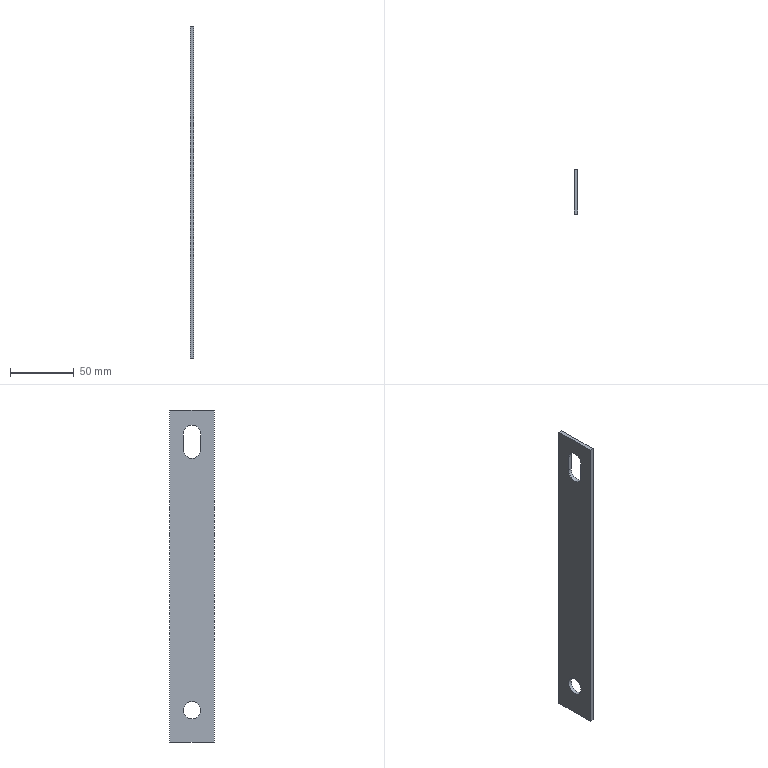Part | NX | features solid 2 | 1 solid | 11 faces | box 3 x 35 x 260 mm | volume 25935 mm3 | plane 8 | cylinder 3 | commonest cylinder face diameters 13.5 x3
STEP:
#1=CARTESIAN_POINT('',(1230.,-511.75,76.25));
#2=VERTEX_POINT('',#1);
#3=CARTESIAN_POINT('',(1230.,-498.25,76.25));
#4=VERTEX_POINT('',#3);
#5=CARTESIAN_POINT('',(1230.,-505.,76.25));
#6=DIRECTION('',(-1.,0.,0.));
#7=DIRECTION('',(0.,-1.,0.));
#8=AXIS2_PLACEMENT_3D('',#5,#6,#7);
#9=CIRCLE('',#8,6.75);
#10=EDGE_CURVE('',#2,#4,#9,.T.);
#11=ORIENTED_EDGE('',*,*,#10,.T.);
#12=CARTESIAN_POINT('',(1233.,-498.25,76.25));
#13=VERTEX_POINT('',#12);
#14=CARTESIAN_POINT('',(1233.,-498.25,76.25));
#15=DIRECTION('',(-1.,0.,0.));
#16=VECTOR('',#15,1000.);
#17=LINE('',#14,#16);
#18=EDGE_CURVE('',#13,#4,#17,.T.);
#19=ORIENTED_EDGE('',*,*,#18,.F.);
#20=CARTESIAN_POINT('',(1233.,-511.75,76.25));
#21=VERTEX_POINT('',#20);
#22=CARTESIAN_POINT('',(1233.,-505.,76.25));
#23=DIRECTION('',(-1.,0.,0.));
#24=DIRECTION('',(0.,-1.,0.));
#25=AXIS2_PLACEMENT_3D('',#22,#23,#24);
#26=CIRCLE('',#25,6.75);
#27=EDGE_CURVE('',#21,#13,#26,.T.);
#28=ORIENTED_EDGE('',*,*,#27,.F.);
#29=CARTESIAN_POINT('',(1233.,-511.75,76.25));
#30=DIRECTION('',(-1.,0.,0.));
#31=VECTOR('',#30,1000.);
#32=LINE('',#29,#31);
#33=EDGE_CURVE('',#21,#2,#32,.T.);
#34=ORIENTED_EDGE('',*,*,#33,.T.);
#35=EDGE_LOOP('',(#11,#19,#28,#34));
#36=FACE_BOUND('',#35,.T.);
#37=CARTESIAN_POINT('',(1233.,-505.,76.25));
#38=DIRECTION('',(-1.,0.,0.));
#39=DIRECTION('',(0.,-1.,0.));
#40=AXIS2_PLACEMENT_3D('',#37,#38,#39);
#41=CYLINDRICAL_SURFACE('',#40,6.75);
#42=ADVANCED_FACE('',(#36),#41,.F.);
#43=CARTESIAN_POINT('',(1230.,-511.75,63.75));
#44=VERTEX_POINT('',#43);
#45=CARTESIAN_POINT('',(1230.,-511.75,76.25));
#46=DIRECTION('',(0.,0.,-1.));
#47=VECTOR('',#46,1000.);
#48=LINE('',#45,#47);
#49=EDGE_CURVE('',#2,#44,#48,.T.);
#50=ORIENTED_EDGE('',*,*,#49,.F.);
#51=ORIENTED_EDGE('',*,*,#33,.F.);
#52=CARTESIAN_POINT('',(1233.,-511.75,63.75));
#53=VERTEX_POINT('',#52);
#54=CARTESIAN_POINT('',(1233.,-511.75,76.25));
#55=DIRECTION('',(0.,0.,-1.));
#56=VECTOR('',#55,1000.);
#57=LINE('',#54,#56);
#58=EDGE_CURVE('',#21,#53,#57,.T.);
#59=ORIENTED_EDGE('',*,*,#58,.T.);
#60=CARTESIAN_POINT('',(1233.,-511.75,63.75));
#61=DIRECTION('',(-1.,0.,0.));
#62=VECTOR('',#61,1000.);
#63=LINE('',#60,#62);
#64=EDGE_CURVE('',#53,#44,#63,.T.);
#65=ORIENTED_EDGE('',*,*,#64,.T.);
#66=EDGE_LOOP('',(#50,#51,#59,#65));
#67=FACE_BOUND('',#66,.T.);
#68=CARTESIAN_POINT('',(1233.,-511.75,76.25));
#69=DIRECTION('',(0.,1.,0.));
#70=DIRECTION('',(-1.,0.,0.));
#71=AXIS2_PLACEMENT_3D('',#68,#69,#70);
#72=PLANE('',#71);
#73=ADVANCED_FACE('',(#67),#72,.T.);
#74=CARTESIAN_POINT('',(1230.,-498.25,63.75));
#75=VERTEX_POINT('',#74);
#76=CARTESIAN_POINT('',(1230.,-505.,63.75));
#77=DIRECTION('',(-1.,0.,0.));
#78=DIRECTION('',(0.,-1.,0.));
#79=AXIS2_PLACEMENT_3D('',#76,#77,#78);
#80=CIRCLE('',#79,6.75);
#81=EDGE_CURVE('',#75,#44,#80,.T.);
#82=ORIENTED_EDGE('',*,*,#81,.T.);
#83=ORIENTED_EDGE('',*,*,#64,.F.);
#84=CARTESIAN_POINT('',(1233.,-498.25,63.75));
#85=VERTEX_POINT('',#84);
#86=CARTESIAN_POINT('',(1233.,-505.,63.75));
#87=DIRECTION('',(-1.,0.,0.));
#88=DIRECTION('',(0.,-1.,0.));
#89=AXIS2_PLACEMENT_3D('',#86,#87,#88);
#90=CIRCLE('',#89,6.75);
#91=EDGE_CURVE('',#85,#53,#90,.T.);
#92=ORIENTED_EDGE('',*,*,#91,.F.);
#93=CARTESIAN_POINT('',(1233.,-498.25,63.75));
#94=DIRECTION('',(-1.,0.,0.));
#95=VECTOR('',#94,1000.);
#96=LINE('',#93,#95);
#97=EDGE_CURVE('',#85,#75,#96,.T.);
#98=ORIENTED_EDGE('',*,*,#97,.T.);
#99=EDGE_LOOP('',(#82,#83,#92,#98));
#100=FACE_BOUND('',#99,.T.);
#101=CARTESIAN_POINT('',(1233.,-505.,63.75));
#102=DIRECTION('',(-1.,0.,0.));
#103=DIRECTION('',(0.,-1.,0.));
#104=AXIS2_PLACEMENT_3D('',#101,#102,#103);
#105=CYLINDRICAL_SURFACE('',#104,6.75);
#106=ADVANCED_FACE('',(#100),#105,.F.);
#107=CARTESIAN_POINT('',(1230.,-522.5,-165.));
#108=VERTEX_POINT('',#107);
#109=CARTESIAN_POINT('',(1230.,-522.5,95.));
#110=VERTEX_POINT('',#109);
#111=CARTESIAN_POINT('',(1230.,-522.5,-205.));
#112=DIRECTION('',(0.,0.,1.));
#113=VECTOR('',#112,1000.);
#114=LINE('',#111,#113);
#115=EDGE_CURVE('',#108,#110,#114,.T.);
#116=ORIENTED_EDGE('',*,*,#115,.F.);
#117=CARTESIAN_POINT('',(1233.,-522.5,-165.));
#118=VERTEX_POINT('',#117);
#119=CARTESIAN_POINT('',(1233.,-522.5,-165.));
#120=DIRECTION('',(-1.,0.,0.));
#121=VECTOR('',#120,1000.);
#122=LINE('',#119,#121);
#123=EDGE_CURVE('',#118,#108,#122,.T.);
#124=ORIENTED_EDGE('',*,*,#123,.F.);
#125=CARTESIAN_POINT('',(1233.,-522.5,95.));
#126=VERTEX_POINT('',#125);
#127=CARTESIAN_POINT('',(1233.,-522.5,-205.));
#128=DIRECTION('',(0.,0.,1.));
#129=VECTOR('',#128,1000.);
#130=LINE('',#127,#129);
#131=EDGE_CURVE('',#118,#126,#130,.T.);
#132=ORIENTED_EDGE('',*,*,#131,.T.);
#133=CARTESIAN_POINT('',(1233.,-522.5,95.));
#134=DIRECTION('',(-1.,0.,0.));
#135=VECTOR('',#134,1000.);
#136=LINE('',#133,#135);
#137=EDGE_CURVE('',#126,#110,#136,.T.);
#138=ORIENTED_EDGE('',*,*,#137,.T.);
#139=EDGE_LOOP('',(#116,#124,#132,#138));
#140=FACE_BOUND('',#139,.T.);
#141=CARTESIAN_POINT('',(1233.,-522.5,-205.));
#142=DIRECTION('',(0.,-1.,0.));
#143=DIRECTION('',(0.,0.,1.));
#144=AXIS2_PLACEMENT_3D('',#141,#142,#143);
#145=PLANE('',#144);
#146=ADVANCED_FACE('',(#140),#145,.T.);
#147=CARTESIAN_POINT('',(1230.,-487.5,95.));
#148=VERTEX_POINT('',#147);
#149=CARTESIAN_POINT('',(1230.,-522.5,95.));
#150=DIRECTION('',(0.,1.,0.));
#151=VECTOR('',#150,1000.);
#152=LINE('',#149,#151);
#153=EDGE_CURVE('',#110,#148,#152,.T.);
#154=ORIENTED_EDGE('',*,*,#153,.F.);
#155=ORIENTED_EDGE('',*,*,#137,.F.);
#156=CARTESIAN_POINT('',(1233.,-487.5,95.));
#157=VERTEX_POINT('',#156);
#158=CARTESIAN_POINT('',(1233.,-522.5,95.));
#159=DIRECTION('',(0.,1.,0.));
#160=VECTOR('',#159,1000.);
#161=LINE('',#158,#160);
#162=EDGE_CURVE('',#126,#157,#161,.T.);
#163=ORIENTED_EDGE('',*,*,#162,.T.);
#164=CARTESIAN_POINT('',(1233.,-487.5,95.));
#165=DIRECTION('',(-1.,0.,0.));
#166=VECTOR('',#165,1000.);
#167=LINE('',#164,#166);
#168=EDGE_CURVE('',#157,#148,#167,.T.);
#169=ORIENTED_EDGE('',*,*,#168,.T.);
#170=EDGE_LOOP('',(#154,#155,#163,#169));
#171=FACE_BOUND('',#170,.T.);
#172=CARTESIAN_POINT('',(1233.,-522.5,95.));
#173=DIRECTION('',(0.,0.,1.));
#174=DIRECTION('',(-1.,0.,0.));
#175=AXIS2_PLACEMENT_3D('',#172,#173,#174);
#176=PLANE('',#175);
#177=ADVANCED_FACE('',(#171),#176,.T.);
#178=CARTESIAN_POINT('',(1230.,-487.5,-165.));
#179=VERTEX_POINT('',#178);
#180=CARTESIAN_POINT('',(1230.,-487.5,95.));
#181=DIRECTION('',(0.,0.,-1.));
#182=VECTOR('',#181,1000.);
#183=LINE('',#180,#182);
#184=EDGE_CURVE('',#148,#179,#183,.T.);
#185=ORIENTED_EDGE('',*,*,#184,.F.);
#186=ORIENTED_EDGE('',*,*,#168,.F.);
#187=CARTESIAN_POINT('',(1233.,-487.5,-165.));
#188=VERTEX_POINT('',#187);
#189=CARTESIAN_POINT('',(1233.,-487.5,95.));
#190=DIRECTION('',(0.,0.,-1.));
#191=VECTOR('',#190,1000.);
#192=LINE('',#189,#191);
#193=EDGE_CURVE('',#157,#188,#192,.T.);
#194=ORIENTED_EDGE('',*,*,#193,.T.);
#195=CARTESIAN_POINT('',(1233.,-487.5,-165.));
#196=DIRECTION('',(-1.,0.,0.));
#197=VECTOR('',#196,1000.);
#198=LINE('',#195,#197);
#199=EDGE_CURVE('',#188,#179,#198,.T.);
#200=ORIENTED_EDGE('',*,*,#199,.T.);
#201=EDGE_LOOP('',(#185,#186,#194,#200));
#202=FACE_BOUND('',#201,.T.);
#203=CARTESIAN_POINT('',(1233.,-487.5,95.));
#204=DIRECTION('',(0.,1.,0.));
#205=DIRECTION('',(0.,0.,-1.));
#206=AXIS2_PLACEMENT_3D('',#203,#204,#205);
#207=PLANE('',#206);
#208=ADVANCED_FACE('',(#202),#207,.T.);
#209=CARTESIAN_POINT('',(1233.,-511.75,-140.));
#210=VERTEX_POINT('',#209);
#211=CARTESIAN_POINT('',(1233.,-505.,-140.));
#212=DIRECTION('',(-1.,0.,0.));
#213=DIRECTION('',(0.,-1.,0.));
#214=AXIS2_PLACEMENT_3D('',#211,#212,#213);
#215=CIRCLE('',#214,6.75);
#216=EDGE_CURVE('',#210,#210,#215,.T.);
#217=ORIENTED_EDGE('',*,*,#216,.F.);
#218=EDGE_LOOP('',(#217));
#219=FACE_BOUND('',#218,.T.);
#220=CARTESIAN_POINT('',(1230.,-511.75,-140.));
#221=VERTEX_POINT('',#220);
#222=CARTESIAN_POINT('',(1230.,-505.,-140.));
#223=DIRECTION('',(-1.,0.,0.));
#224=DIRECTION('',(0.,-1.,0.));
#225=AXIS2_PLACEMENT_3D('',#222,#223,#224);
#226=CIRCLE('',#225,6.75);
#227=EDGE_CURVE('',#221,#221,#226,.T.);
#228=ORIENTED_EDGE('',*,*,#227,.T.);
#229=EDGE_LOOP('',(#228));
#230=FACE_BOUND('',#229,.T.);
#231=CARTESIAN_POINT('',(1233.,-505.,-140.));
#232=DIRECTION('',(-1.,0.,0.));
#233=DIRECTION('',(0.,-1.,0.));
#234=AXIS2_PLACEMENT_3D('',#231,#232,#233);
#235=CYLINDRICAL_SURFACE('',#234,6.75);
#236=ADVANCED_FACE('',(#219,#230),#235,.F.);
#237=CARTESIAN_POINT('',(1230.,-522.5,-165.));
#238=DIRECTION('',(0.,-1.,0.));
#239=VECTOR('',#238,1000.);
#240=LINE('',#237,#239);
#241=EDGE_CURVE('',#179,#108,#240,.T.);
#242=ORIENTED_EDGE('',*,*,#241,.F.);
#243=ORIENTED_EDGE('',*,*,#199,.F.);
#244=CARTESIAN_POINT('',(1233.,-522.5,-165.));
#245=DIRECTION('',(0.,-1.,0.));
#246=VECTOR('',#245,1000.);
#247=LINE('',#244,#246);
#248=EDGE_CURVE('',#188,#118,#247,.T.);
#249=ORIENTED_EDGE('',*,*,#248,.T.);
#250=ORIENTED_EDGE('',*,*,#123,.T.);
#251=EDGE_LOOP('',(#242,#243,#249,#250));
#252=FACE_BOUND('',#251,.T.);
#253=CARTESIAN_POINT('',(1233.,-487.5,-165.));
#254=DIRECTION('',(0.,0.,-1.));
#255=DIRECTION('',(1.,0.,0.));
#256=AXIS2_PLACEMENT_3D('',#253,#254,#255);
#257=PLANE('',#256);
#258=ADVANCED_FACE('',(#252),#257,.T.);
#259=CARTESIAN_POINT('',(1230.,-498.25,63.75));
#260=DIRECTION('',(0.,0.,1.));
#261=VECTOR('',#260,1000.);
#262=LINE('',#259,#261);
#263=EDGE_CURVE('',#75,#4,#262,.T.);
#264=ORIENTED_EDGE('',*,*,#263,.F.);
#265=ORIENTED_EDGE('',*,*,#97,.F.);
#266=CARTESIAN_POINT('',(1233.,-498.25,63.75));
#267=DIRECTION('',(0.,0.,1.));
#268=VECTOR('',#267,1000.);
#269=LINE('',#266,#268);
#270=EDGE_CURVE('',#85,#13,#269,.T.);
#271=ORIENTED_EDGE('',*,*,#270,.T.);
#272=ORIENTED_EDGE('',*,*,#18,.T.);
#273=EDGE_LOOP('',(#264,#265,#271,#272));
#274=FACE_BOUND('',#273,.T.);
#275=CARTESIAN_POINT('',(1233.,-498.25,63.75));
#276=DIRECTION('',(0.,-1.,0.));
#277=DIRECTION('',(1.,0.,0.));
#278=AXIS2_PLACEMENT_3D('',#275,#276,#277);
#279=PLANE('',#278);
#280=ADVANCED_FACE('',(#274),#279,.T.);
#281=ORIENTED_EDGE('',*,*,#131,.F.);
#282=ORIENTED_EDGE('',*,*,#248,.F.);
#283=ORIENTED_EDGE('',*,*,#193,.F.);
#284=ORIENTED_EDGE('',*,*,#162,.F.);
#285=EDGE_LOOP('',(#281,#282,#283,#284));
#286=FACE_BOUND('',#285,.T.);
#287=ORIENTED_EDGE('',*,*,#216,.T.);
#288=EDGE_LOOP('',(#287));
#289=FACE_BOUND('',#288,.T.);
#290=ORIENTED_EDGE('',*,*,#27,.T.);
#291=ORIENTED_EDGE('',*,*,#270,.F.);
#292=ORIENTED_EDGE('',*,*,#91,.T.);
#293=ORIENTED_EDGE('',*,*,#58,.F.);
#294=EDGE_LOOP('',(#290,#291,#292,#293));
#295=FACE_BOUND('',#294,.T.);
#296=CARTESIAN_POINT('',(1233.,-522.5,95.));
#297=DIRECTION('',(-1.,0.,0.));
#298=DIRECTION('',(0.,-1.,0.));
#299=AXIS2_PLACEMENT_3D('',#296,#297,#298);
#300=PLANE('',#299);
#301=ADVANCED_FACE('',(#286,#289,#295),#300,.F.);
#302=ORIENTED_EDGE('',*,*,#115,.T.);
#303=ORIENTED_EDGE('',*,*,#153,.T.);
#304=ORIENTED_EDGE('',*,*,#184,.T.);
#305=ORIENTED_EDGE('',*,*,#241,.T.);
#306=EDGE_LOOP('',(#302,#303,#304,#305));
#307=FACE_BOUND('',#306,.T.);
#308=ORIENTED_EDGE('',*,*,#227,.F.);
#309=EDGE_LOOP('',(#308));
#310=FACE_BOUND('',#309,.T.);
#311=ORIENTED_EDGE('',*,*,#10,.F.);
#312=ORIENTED_EDGE('',*,*,#49,.T.);
#313=ORIENTED_EDGE('',*,*,#81,.F.);
#314=ORIENTED_EDGE('',*,*,#263,.T.);
#315=EDGE_LOOP('',(#311,#312,#313,#314));
#316=FACE_BOUND('',#315,.T.);
#317=CARTESIAN_POINT('',(1230.,-522.5,95.));
#318=DIRECTION('',(-1.,0.,0.));
#319=DIRECTION('',(0.,-1.,0.));
#320=AXIS2_PLACEMENT_3D('',#317,#318,#319);
#321=PLANE('',#320);
#322=ADVANCED_FACE('',(#307,#310,#316),#321,.T.);
#323=CLOSED_SHELL('',(#42,#73,#106,#146,#177,#208,#236,#258,#280,#301,#322));
#324=MANIFOLD_SOLID_BREP('',#323);
#325=(LENGTH_UNIT()NAMED_UNIT(*)SI_UNIT(.MILLI.,.METRE.));
#326=UNCERTAINTY_MEASURE_WITH_UNIT(LENGTH_MEASURE(0.00001),#325,'','');
#327=(NAMED_UNIT(*)PLANE_ANGLE_UNIT()SI_UNIT($,.RADIAN.));
#328=(NAMED_UNIT(*)SI_UNIT($,.STERADIAN.)SOLID_ANGLE_UNIT());
#329=(GEOMETRIC_REPRESENTATION_CONTEXT(3)GLOBAL_UNCERTAINTY_ASSIGNED_CONTEXT((#326))GLOBAL_UNIT_ASSIGNED_CONTEXT((#325,#327,#328))REPRESENTATION_CONTEXT('',''));
#330=ADVANCED_BREP_SHAPE_REPRESENTATION('',(#324),#329);